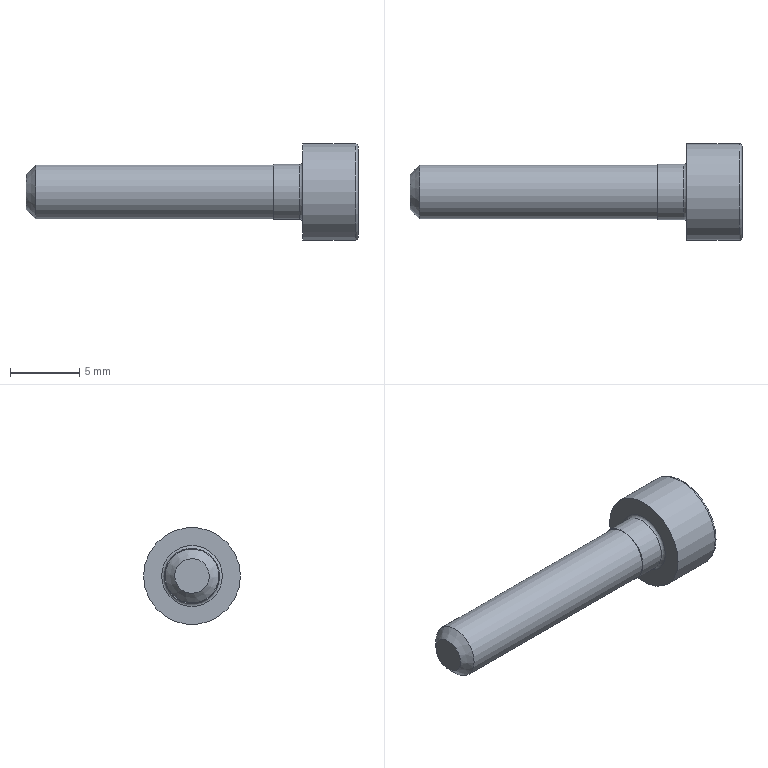Part | STEP file | PARAFUSO M4x20 - DIN_912 | 1 solid | 24 faces | box 24 x 7 x 7 mm | volume 373.112 mm3 | plane 11 | cylinder 9 | torus 2 | cone 2 | commonest cylinder face diameters 3.443 x6 3.902 x1 4 x1 7 x1